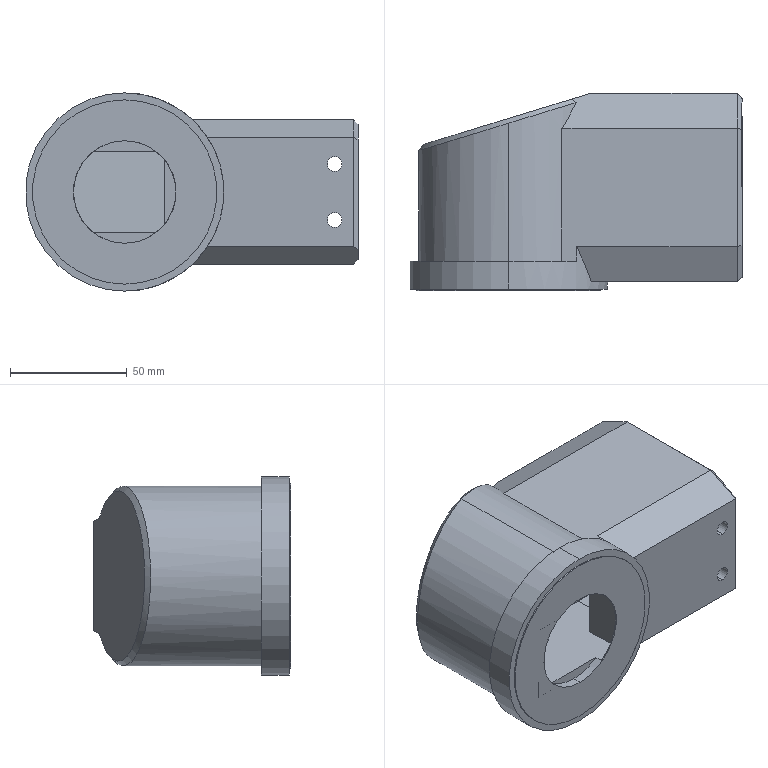Part | SolidWorks | features BaseBody 1 | 1 solid | 62 faces | box 142.5 x 84.5 x 85 mm | volume 371166 mm3 | plane 40 | cylinder 21 | spline 1 | commonest cylinder face diameters 6.2 x12 77 x3 44 x2 79 x2 85 x2